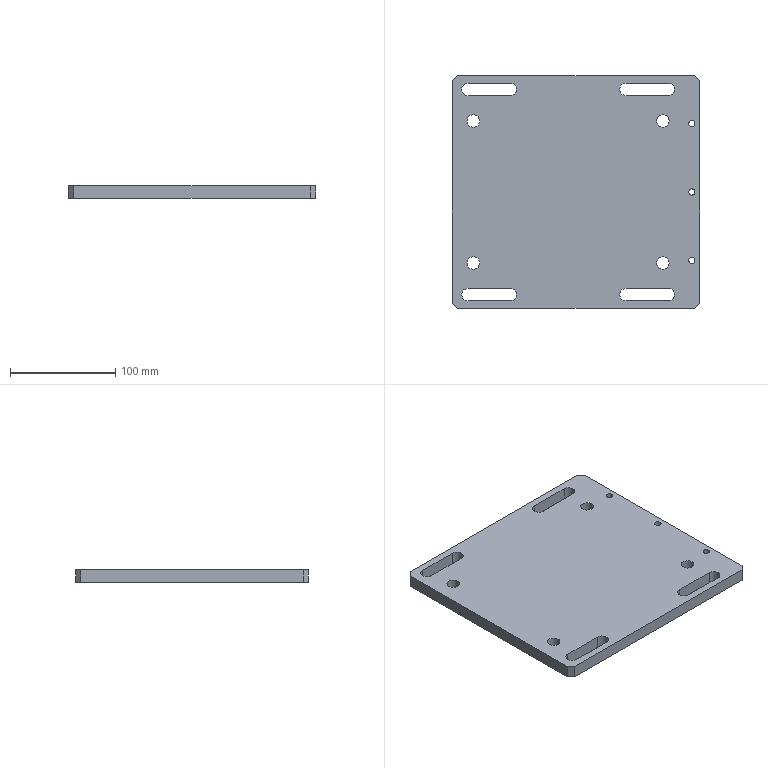Part | STEP file | MOTOR.BASE.stp | 1 solid | 42 faces | box 235 x 221 x 12 mm | volume 587706 mm3 | cylinder 18 | plane 13 | spline 11 | commonest cylinder face diameters 12 x14 6 x4